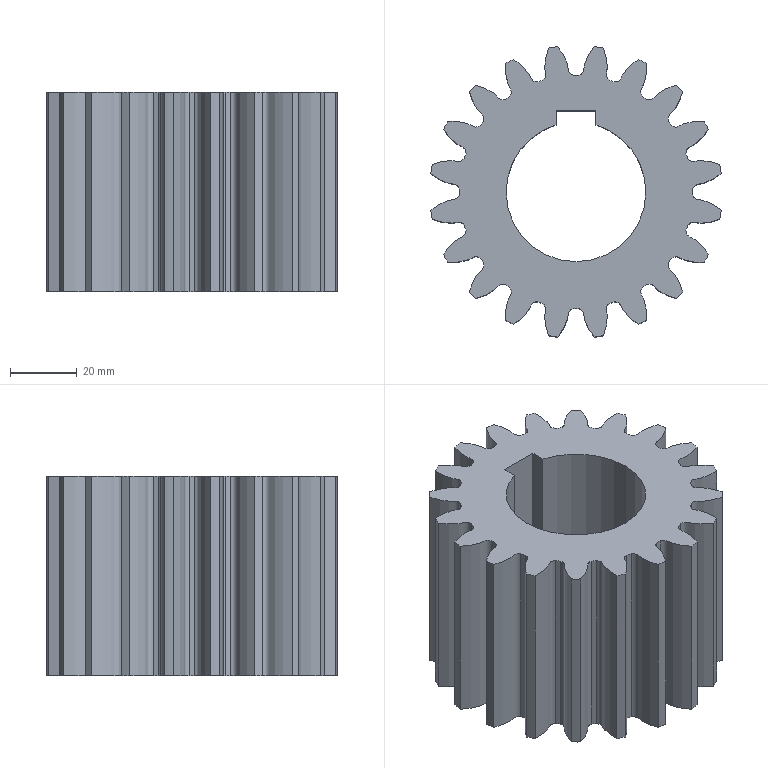Part | SolidWorks | features BaseBody 1 | 1 solid | 89 faces | box 87.307 x 87.307 x 60 mm | volume 210488 mm3 | cylinder 44 | spline 40 | plane 5 | commonest cylinder face diameters 70 x21 88 x20 42 x3